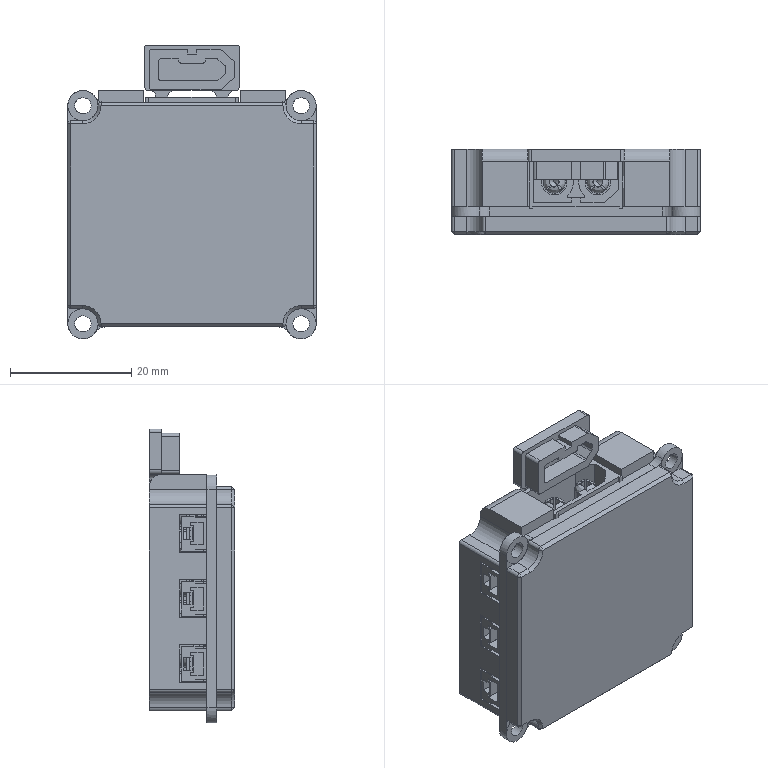Part | SolidWorks | features BaseBody 37 | 37 solids | 4985 faces | volume 15304 mm3 | plane 3072 | cylinder 1445 | spline 248 | cone 220 | commonest cylinder face diameters 2.5 x128 1 x110 2 x101 0.8 x98 1.6 x58 3 x58